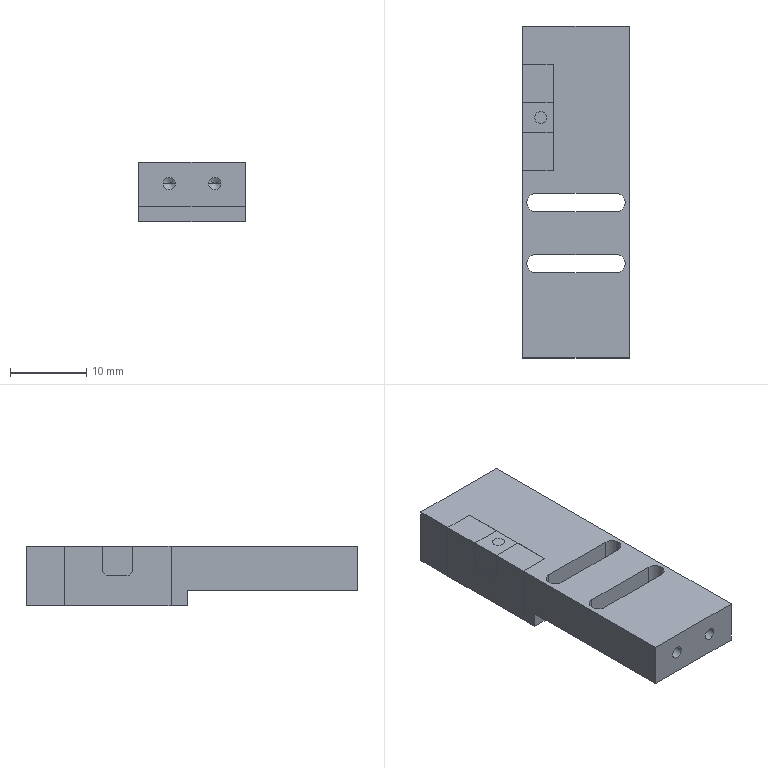Part | 2 solids | 70 faces | box 14 x 43.5 x 7.8 mm | volume 3729 mm3 | plane 28 | cylinder 24 | cone 18 | commonest cylinder face diameters 1.6 x14 2 x6 2.4 x4